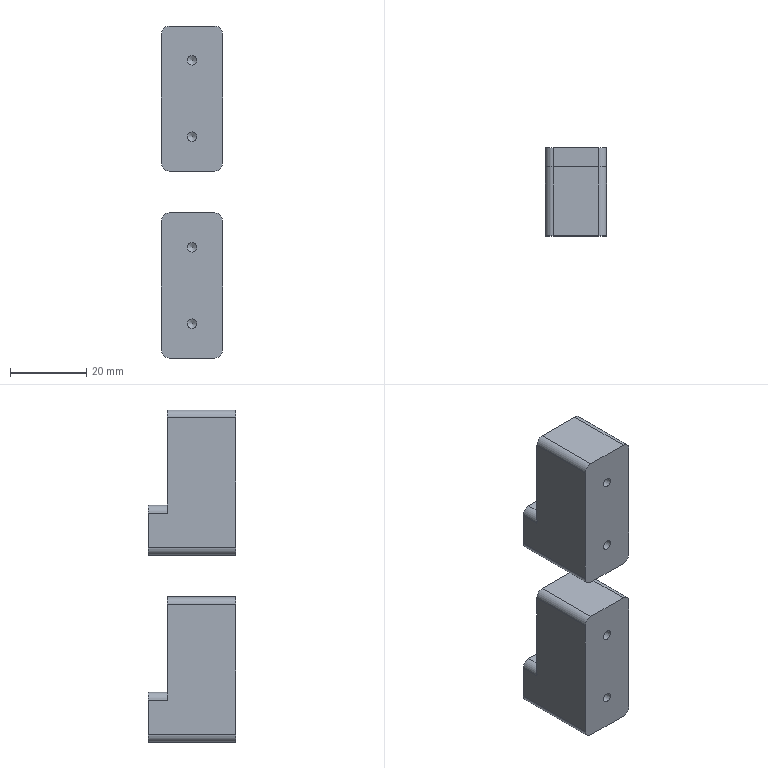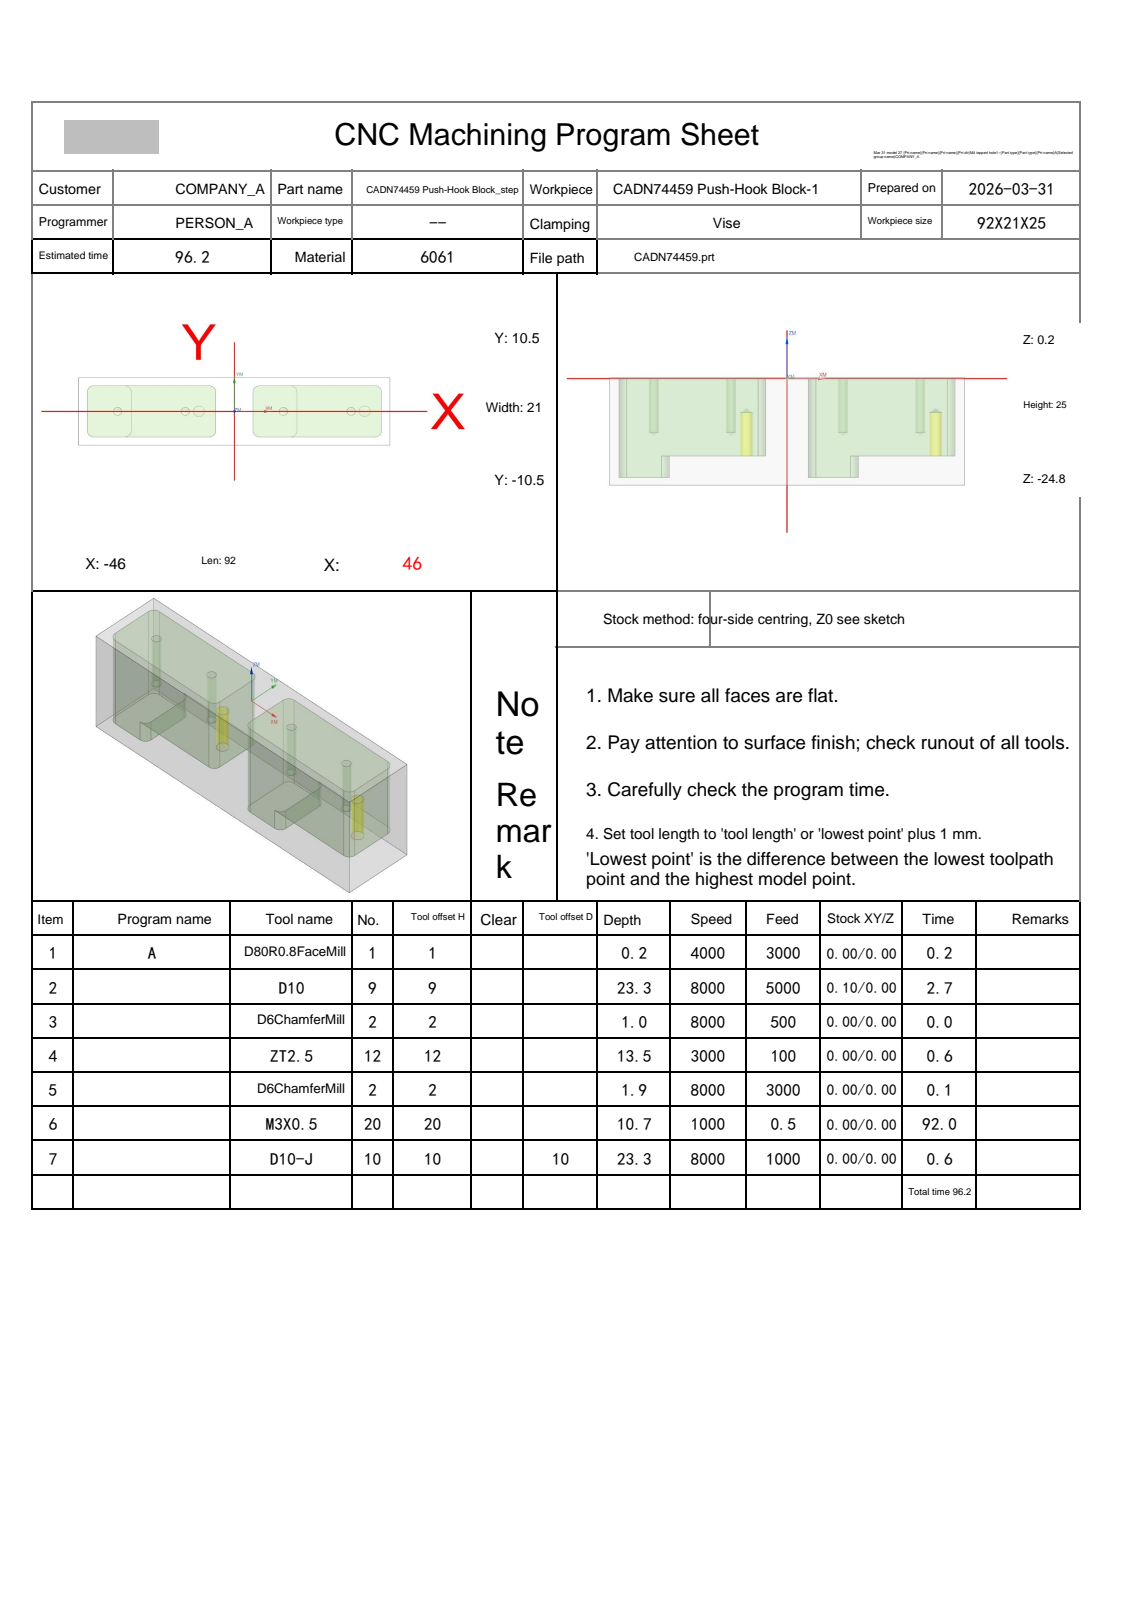NC program | NX | posted by the shop | part box 16 x 23 x 87 mm
Whole program:
%
O0001
(Machine time: 181.72 MIN)
(===Total Tool:6===)
(T1=D80R0.8 Mill D=80.  R=0.8  D-  H01 Z=0.    )
(T9=D10     D=10.  R=0.   D-  H09 Z=-23.1 )
(T2=D6ChamferMill   D=6.   R=0.   D-  H02 Z=-1.75 )
(T12=ZT2.5  D=2.5  DR_a=118 D-  H12 Z=-13.25)
(T20=M3X0.5 D=2.5  DR_a=180 D-  H20 Z=-10.5 )
(T10=D10-J  D=10.  R=0.   D10 H10 Z=-23.1 )
G80 G90 G17 G49 G40
G91 G28 Z0
M01
N1 T01 M06
(D80R0.8 Mill  D=80. R=0.8 H=01 ce=0.20 di=0.10)
G00 G90 G54 X-88.5 Y0.0 M03 S4000
G43 H01 Z20.
M08
Z2.1
G01 Z.1 F3000.
X-83.5
X83.5
X88.5
Z2.1
G00 Z20.
G00 G90 X-88.5 Y0.0 M03 S4000
Z20.
Z2.
G01 Z0.0 F1000.
X-83.5
X83.5
X88.5
Z2.
G00 Z20.
G91 G28 Z0.0
M05
M09
G91 G28 Z0.0
M01
N2 T09 M06
(D10  D=10. R=0. H=09 ce=0.10 di=0.00)
G00 G90 G54 X24.5 Y13.1 M03 S8000
G43 H09 Z20.
M08
Z.5
G01 X41.5 Z.439 F5000.
G02 X48.6 Y6. Z.399 I0.0 J-7.1
G01 Y-6. Z.355
G02 X41.5 Y-13.1 Z.315 I-7.1 J0.0
G01 X7.5 Z.193
G02 X.4 Y-6. Z.153 I0.0 J7.1
G01 Y6. Z.11
G02 X7.5 Y13.1 Z.07 I7.1 J0.0
G01 X41.5 Z-.053
G02 X48.6 Y6. Z-.093 I0.0 J-7.1
G01 Y-6. Z-.136
G02 X41.5 Y-13.1 Z-.176 I-7.1 J0.0
G01 X7.5 Z-.299
G02 X.4 Y-6. Z-.339 I0.0 J7.1
G01 Y6. Z-.382
G02 X7.5 Y13.1 Z-.422 I7.1 J0.0
G01 X41.5 Z-.545
G02 X48.6 Y6. Z-.585 I0.0 J-7.1
G01 Y-6. Z-.628
G02 X41.5 Y-13.1 Z-.668 I-7.1 J0.0
G01 X7.5 Z-.79
G02 X.4 Y-6. Z-.83 I0.0 J7.1
G01 Y6. Z-.874
G02 X7.5 Y13.1 Z-.914 I7.1 J0.0
G01 X41.5 Z-1.036
G02 X48.6 Y6. Z-1.076 I0.0 J-7.1
G01 Y-6. Z-1.12
G02 X41.5 Y-13.1 Z-1.16 I-7.1 J0.0
G01 X7.5 Z-1.282
G02 X.4 Y-6. Z-1.322 I0.0 J7.1
G01 Y6. Z-1.365
G02 X7.5 Y13.1 Z-1.405 I7.1 J0.0
G01 X41.5 Z-1.528
G02 X48.6 Y6. Z-1.568 I0.0 J-7.1
G01 Y-6. Z-1.611
G02 X41.5 Y-13.1 Z-1.651 I-7.1 J0.0
G01 X7.5 Z-1.774
G02 X.4 Y-6. Z-1.814 I0.0 J7.1
G01 Y6. Z-1.857
G02 X7.5 Y13.1 Z-1.897 I7.1 J0.0
G01 X41.5 Z-2.02
G02 X48.6 Y6. Z-2.06 I0.0 J-7.1
G01 Y-6. Z-2.103
G02 X41.5 Y-13.1 Z-2.143 I-7.1 J0.0
G01 X7.5 Z-2.265
G02 X.4 Y-6. Z-2.305 I0.0 J7.1
G01 Y6. Z-2.349
G02 X7.5 Y13.1 Z-2.389 I7.1 J0.0
G01 X41.5 Z-2.511
G02 X48.6 Y6. Z-2.551 I0.0 J-7.1
G01 Y-6. Z-2.595
G02 X41.5 Y-13.1 Z-2.635 I-7.1 J0.0
G01 X7.5 Z-2.757
G02 X.4 Y-6. Z-2.797 I0.0 J7.1
G01 Y6. Z-2.84
G02 X7.5 Y13.1 Z-2.88 I7.1 J0.0
G01 X41.5 Z-3.003
G02 X48.6 Y6. Z-3.043 I0.0 J-7.1
G01 Y-6. Z-3.086
G02 X41.5 Y-13.1 Z-3.126 I-7.1 J0.0
G01 X7.5 Z-3.249
G02 X.4 Y-6. Z-3.289 I0.0 J7.1
G01 Y6. Z-3.332
G02 X7.5 Y13.1 Z-3.372 I7.1 J0.0
G01 X41.5 Z-3.495
G02 X48.6 Y6. Z-3.535 I0.0 J-7.1
G01 Y-6. Z-3.578
G02 X41.5 Y-13.1 Z-3.618 I-7.1 J0.0
G01 X7.5 Z-3.74
G02 X.4 Y-6. Z-3.78 I0.0 J7.1
G01 Y6. Z-3.824
G02 X7.5 Y13.1 Z-3.864 I7.1 J0.0
G01 X41.5 Z-3.986
G02 X48.6 Y6. Z-4.026 I0.0 J-7.1
G01 Y-6. Z-4.07
G02 X41.5 Y-13.1 Z-4.11 I-7.1 J0.0
G01 X7.5 Z-4.232
G02 X.4 Y-6. Z-4.272 I0.0 J7.1
G01 Y6. Z-4.315
G02 X7.5 Y13.1 Z-4.355 I7.1 J0.0
G01 X41.5 Z-4.478
G02 X48.6 Y6. Z-4.518 I0.0 J-7.1
G01 Y-6. Z-4.561
G02 X41.5 Y-13.1 Z-4.601 I-7.1 J0.0
G01 X7.5 Z-4.724
G02 X.4 Y-6. Z-4.764 I0.0 J7.1
G01 Y6. Z-4.807
G02 X7.5 Y13.1 Z-4.847 I7.1 J0.0
G01 X41.5 Z-4.97
G02 X48.6 Y6. Z-5.01 I0.0 J-7.1
G01 Y-6. Z-5.053
G02 X41.5 Y-13.1 Z-5.093 I-7.1 J0.0
G01 X7.5 Z-5.215
G02 X.4 Y-6. Z-5.255 I0.0 J7.1
G01 Y6. Z-5.299
G02 X7.5 Y13.1 Z-5.339 I7.1 J0.0
G01 X41.5 Z-5.461
G02 X48.6 Y6. Z-5.501 I0.0 J-7.1
G01 Y-6. Z-5.545
G02 X41.5 Y-13.1 Z-5.585 I-7.1 J0.0
G01 X7.5 Z-5.707
G02 X.4 Y-6. Z-5.747 I0.0 J7.1
G01 Y6. Z-5.79
G02 X7.5 Y13.1 Z-5.83 I7.1 J0.0
G01 X41.5 Z-5.953
G02 X48.6 Y6. Z-5.993 I0.0 J-7.1
G01 Y-6. Z-6.036
G02 X41.5 Y-13.1 Z-6.076 I-7.1 J0.0
G01 X7.5 Z-6.199
G02 X.4 Y-6. Z-6.239 I0.0 J7.1
G01 Y6. Z-6.282
G02 X7.5 Y13.1 Z-6.322 I7.1 J0.0
G01 X41.5 Z-6.445
G02 X48.6 Y6. Z-6.485 I0.0 J-7.1
G01 Y-6. Z-6.528
G02 X41.5 Y-13.1 Z-6.568 I-7.1 J0.0
G01 X7.5 Z-6.69
G02 X.4 Y-6. Z-6.73 I0.0 J7.1
G01 Y6. Z-6.774
G02 X7.5 Y13.1 Z-6.814 I7.1 J0.0
G01 X41.5 Z-6.936
G02 X48.6 Y6. Z-6.976 I0.0 J-7.1
G01 Y-6. Z-7.02
G02 X41.5 Y-13.1 Z-7.06 I-7.1 J0.0
G01 X7.5 Z-7.182
G02 X.4 Y-6. Z-7.222 I0.0 J7.1
G01 Y6. Z-7.265
G02 X7.5 Y13.1 Z-7.305 I7.1 J0.0
G01 X41.5 Z-7.428
G02 X48.6 Y6. Z-7.468 I0.0 J-7.1
G01 Y-6. Z-7.511
G02 X41.5 Y-13.1 Z-7.551 I-7.1 J0.0
G01 X7.5 Z-7.674
G02 X.4 Y-6. Z-7.714 I0.0 J7.1
G01 Y6. Z-7.757
G02 X7.5 Y13.1 Z-7.797 I7.1 J0.0
G01 X41.5 Z-7.92
G02 X48.6 Y6. Z-7.96 I0.0 J-7.1
G01 Y-6. Z-8.003
G02 X41.5 Y-13.1 Z-8.043 I-7.1 J0.0
G01 X7.5 Z-8.165
G02 X.4 Y-6. Z-8.205 I0.0 J7.1
G01 Y6. Z-8.249
G02 X7.5 Y13.1 Z-8.289 I7.1 J0.0
G01 X41.5 Z-8.411
G02 X48.6 Y6. Z-8.451 I0.0 J-7.1
G01 Y-6. Z-8.495
G02 X41.5 Y-13.1 Z-8.535 I-7.1 J0.0
G01 X7.5 Z-8.657
G02 X.4 Y-6. Z-8.697 I0.0 J7.1
G01 Y6. Z-8.74
G02 X7.5 Y13.1 Z-8.78 I7.1 J0.0
G01 X41.5 Z-8.903
G02 X48.6 Y6. Z-8.943 I0.0 J-7.1
G01 Y-6. Z-8.986
G02 X41.5 Y-13.1 Z-9.026 I-7.1 J0.0
G01 X7.5 Z-9.149
G02 X.4 Y-6. Z-9.189 I0.0 J7.1
G01 Y6. Z-9.232
G02 X7.5 Y13.1 Z-9.272 I7.1 J0.0
G01 X41.5 Z-9.395
G02 X48.6 Y6. Z-9.435 I0.0 J-7.1
G01 Y-6. Z-9.478
G02 X41.5 Y-13.1 Z-9.518 I-7.1 J0.0
G01 X7.5 Z-9.64
G02 X.4 Y-6. Z-9.68 I0.0 J7.1
G01 Y6. Z-9.724
G02 X7.5 Y13.1 Z-9.764 I7.1 J0.0
G01 X41.5 Z-9.886
G02 X48.6 Y6. Z-9.926 I0.0 J-7.1
G01 Y-6. Z-9.97
G02 X41.5 Y-13.1 Z-10.01 I-7.1 J0.0
G01 X7.5 Z-10.132
G02 X.4 Y-6. Z-10.172 I0.0 J7.1
G01 Y6. Z-10.215
G02 X7.5 Y13.1 Z-10.255 I7.1 J0.0
G01 X41.5 Z-10.378
G02 X48.6 Y6. Z-10.418 I0.0 J-7.1
G01 Y-6. Z-10.461
G02 X41.5 Y-13.1 Z-10.501 I-7.1 J0.0
G01 X7.5 Z-10.624
G02 X.4 Y-6. Z-10.664 I0.0 J7.1
G01 Y6. Z-10.707
G02 X7.5 Y13.1 Z-10.747 I7.1 J0.0
G01 X41.5 Z-10.87
G02 X48.6 Y6. Z-10.91 I0.0 J-7.1
G01 Y-6. Z-10.953
G02 X41.5 Y-13.1 Z-10.993 I-7.1 J0.0
G01 X7.5 Z-11.115
G02 X.4 Y-6. Z-11.155 I0.0 J7.1
G01 Y6. Z-11.199
G02 X7.5 Y13.1 Z-11.239 I7.1 J0.0
G01 X41.5 Z-11.361
G02 X48.6 Y6. Z-11.401 I0.0 J-7.1
G01 Y-6. Z-11.445
G02 X41.5 Y-13.1 Z-11.485 I-7.1 J0.0
G01 X7.5 Z-11.607
G02 X.4 Y-6. Z-11.647 I0.0 J7.1
G01 Y6. Z-11.69
G02 X7.5 Y13.1 Z-11.73 I7.1 J0.0
G01 X41.5 Z-11.853
G02 X48.6 Y6. Z-11.893 I0.0 J-7.1
G01 Y-6. Z-11.936
G02 X41.5 Y-13.1 Z-11.976 I-7.1 J0.0
G01 X7.5 Z-12.099
G02 X.4 Y-6. Z-12.139 I0.0 J7.1
G01 Y6. Z-12.182
G02 X7.5 Y13.1 Z-12.222 I7.1 J0.0
G01 X41.5 Z-12.345
G02 X48.6 Y6. Z-12.385 I0.0 J-7.1
G01 Y-6. Z-12.428
G02 X41.5 Y-13.1 Z-12.468 I-7.1 J0.0
G01 X7.5 Z-12.59
G02 X.4 Y-6. Z-12.63 I0.0 J7.1
G01 Y6. Z-12.674
G02 X7.5 Y13.1 Z-12.714 I7.1 J0.0
G01 X41.5 Z-12.836
G02 X48.6 Y6. Z-12.876 I0.0 J-7.1
G01 Y-6. Z-12.92
G02 X41.5 Y-13.1 Z-12.96 I-7.1 J0.0
G01 X7.5 Z-13.082
G02 X.4 Y-6. Z-13.122 I0.0 J7.1
G01 Y6. Z-13.165
G02 X7.5 Y13.1 Z-13.205 I7.1 J0.0
G01 X41.5 Z-13.328
G02 X48.6 Y6. Z-13.368 I0.0 J-7.1
G01 Y-6. Z-13.411
G02 X41.5 Y-13.1 Z-13.451 I-7.1 J0.0
G01 X7.5 Z-13.574
G02 X.4 Y-6. Z-13.614 I0.0 J7.1
G01 Y6. Z-13.657
G02 X7.5 Y13.1 Z-13.697 I7.1 J0.0
G01 X41.5 Z-13.82
G02 X48.6 Y6. Z-13.86 I0.0 J-7.1
G01 Y-6. Z-13.903
G02 X41.5 Y-13.1 Z-13.943 I-7.1 J0.0
G01 X7.5 Z-14.065
G02 X.4 Y-6. Z-14.105 I0.0 J7.1
G01 Y6. Z-14.149
G02 X7.5 Y13.1 Z-14.189 I7.1 J0.0
G01 X41.5 Z-14.311
G02 X48.6 Y6. Z-14.351 I0.0 J-7.1
G01 Y-6. Z-14.395
G02 X41.5 Y-13.1 Z-14.435 I-7.1 J0.0
G01 X7.5 Z-14.557
G02 X.4 Y-6. Z-14.597 I0.0 J7.1
G01 Y6. Z-14.64
G02 X7.5 Y13.1 Z-14.68 I7.1 J0.0
G01 X41.5 Z-14.803
G02 X48.6 Y6. Z-14.843 I0.0 J-7.1
G01 Y-6. Z-14.886
G02 X41.5 Y-13.1 Z-14.926 I-7.1 J0.0
G01 X7.5 Z-15.049
G02 X.4 Y-6. Z-15.089 I0.0 J7.1
G01 Y6. Z-15.132
G02 X7.5 Y13.1 Z-15.172 I7.1 J0.0
G01 X41.5 Z-15.295
G02 X48.6 Y6. Z-15.335 I0.0 J-7.1
G01 Y-6. Z-15.378
G02 X41.5 Y-13.1 Z-15.418 I-7.1 J0.0
G01 X7.5 Z-15.54
G02 X.4 Y-6. Z-15.58 I0.0 J7.1
G01 Y6. Z-15.624
G02 X7.5 Y13.1 Z-15.664 I7.1 J0.0
G01 X41.5 Z-15.786
G02 X48.6 Y6. Z-15.826 I0.0 J-7.1
G01 Y-6. Z-15.87
G02 X41.5 Y-13.1 Z-15.91 I-7.1 J0.0
G01 X7.5 Z-16.032
G02 X.4 Y-6. Z-16.072 I0.0 J7.1
G01 Y6. Z-16.115
G02 X7.5 Y13.1 Z-16.155 I7.1 J0.0
G01 X41.5 Z-16.278
G02 X48.6 Y6. Z-16.318 I0.0 J-7.1
G01 Y-6. Z-16.361
G02 X41.5 Y-13.1 Z-16.401 I-7.1 J0.0
G01 X7.5 Z-16.524
G02 X.4 Y-6. Z-16.564 I0.0 J7.1
G01 Y6. Z-16.607
G02 X7.5 Y13.1 Z-16.647 I7.1 J0.0
G01 X41.5 Z-16.77
G02 X48.6 Y6. Z-16.81 I0.0 J-7.1
G01 Y-6. Z-16.853
G02 X41.5 Y-13.1 Z-16.893 I-7.1 J0.0
G01 X7.5 Z-17.015
G02 X.4 Y-6. Z-17.055 I0.0 J7.1
G01 Y6. Z-17.099
G02 X7.5 Y13.1 Z-17.139 I7.1 J0.0
G01 X41.5 Z-17.261
G02 X48.6 Y6. Z-17.301 I0.0 J-7.1
G01 Y-6. Z-17.345
G02 X41.5 Y-13.1 Z-17.385 I-7.1 J0.0
G01 X7.5 Z-17.507
G02 X.4 Y-6. Z-17.547 I0.0 J7.1
G01 Y6. Z-17.59
G02 X7.5 Y13.1 Z-17.63 I7.1 J0.0
G01 X41.5 Z-17.753
G02 X48.6 Y6. Z-17.793 I0.0 J-7.1
G01 Y-6. Z-17.836
G02 X41.5 Y-13.1 Z-17.876 I-7.1 J0.0
G01 X7.5 Z-17.999
G02 X.4 Y-6. Z-18.039 I0.0 J7.1
G01 Y6. Z-18.082
G02 X7.5 Y13.1 Z-18.122 I7.1 J0.0
G01 X41.5 Z-18.245
G02 X48.6 Y6. Z-18.285 I0.0 J-7.1
G01 Y-6. Z-18.328
G02 X41.5 Y-13.1 Z-18.368 I-7.1 J0.0
G01 X7.5 Z-18.49
G02 X.4 Y-6. Z-18.53 I0.0 J7.1
G01 Y6. Z-18.574
G02 X7.5 Y13.1 Z-18.614 I7.1 J0.0
G01 X41.5 Z-18.736
G02 X48.6 Y6. Z-18.776 I0.0 J-7.1
G01 Y-6. Z-18.82
G02 X41.5 Y-13.1 Z-18.86 I-7.1 J0.0
G01 X7.5 Z-18.982
G02 X.4 Y-6. Z-19.022 I0.0 J7.1
G01 Y6. Z-19.065
G02 X7.5 Y13.1 Z-19.105 I7.1 J0.0
G01 X41.5 Z-19.228
G02 X48.6 Y6. Z-19.268 I0.0 J-7.1
G01 Y-6. Z-19.311
G02 X41.5 Y-13.1 Z-19.351 I-7.1 J0.0
G01 X7.5 Z-19.474
G02 X.4 Y-6. Z-19.514 I0.0 J7.1
G01 Y6. Z-19.557
G02 X7.5 Y13.1 Z-19.597 I7.1 J0.0
G01 X41.5 Z-19.72
G02 X48.6 Y6. Z-19.76 I0.0 J-7.1
G01 Y-6. Z-19.803
G02 X41.5 Y-13.1 Z-19.843 I-7.1 J0.0
G01 X7.5 Z-19.965
G02 X.4 Y-6. Z-20.005 I0.0 J7.1
G01 Y6. Z-20.049
G02 X7.5 Y13.1 Z-20.089 I7.1 J0.0
G01 X41.5 Z-20.211
G02 X48.6 Y6. Z-20.251 I0.0 J-7.1
G01 Y-6. Z-20.295
G02 X41.5 Y-13.1 Z-20.335 I-7.1 J0.0
G01 X7.5 Z-20.457
G02 X.4 Y-6. Z-20.497 I0.0 J7.1
G01 Y6. Z-20.54
G02 X7.5 Y13.1 Z-20.58 I7.1 J0.0
G01 X41.5 Z-20.703
G02 X48.6 Y6. Z-20.743 I0.0 J-7.1
G01 Y-6. Z-20.786
G02 X41.5 Y-13.1 Z-20.826 I-7.1 J0.0
G01 X7.5 Z-20.949
G02 X.4 Y-6. Z-20.989 I0.0 J7.1
G01 Y6. Z-21.032
G02 X7.5 Y13.1 Z-21.072 I7.1 J0.0
G01 X41.5 Z-21.195
G02 X48.6 Y6. Z-21.235 I0.0 J-7.1
G01 Y-6. Z-21.278
G02 X41.5 Y-13.1 Z-21.318 I-7.1 J0.0
G01 X7.5 Z-21.44
G02 X.4 Y-6. Z-21.48 I0.0 J7.1
G01 Y6. Z-21.524
G02 X7.5 Y13.1 Z-21.564 I7.1 J0.0
G01 X41.5 Z-21.686
G02 X48.6 Y6. Z-21.726 I0.0 J-7.1
G01 Y-6. Z-21.77
G02 X41.5 Y-13.1 Z-21.81 I-7.1 J0.0
G01 X7.5 Z-21.932
G02 X.4 Y-6. Z-21.972 I0.0 J7.1
G01 Y6. Z-22.015
G02 X7.5 Y13.1 Z-22.055 I7.1 J0.0
G01 X41.5 Z-22.178
G02 X48.6 Y6. Z-22.218 I0.0 J-7.1
G01 Y-6. Z-22.261
G02 X41.5 Y-13.1 Z-22.301 I-7.1 J0.0
G01 X7.5 Z-22.424
G02 X.4 Y-6. Z-22.464 I0.0 J7.1
G01 Y6. Z-22.507
G02 X7.5 Y13.1 Z-22.547 I7.1 J0.0
G01 X41.5 Z-22.67
G02 X48.6 Y6. Z-22.71 I0.0 J-7.1
G01 Y-6. Z-22.753
G02 X41.5 Y-13.1 Z-22.793 I-7.1 J0.0
G01 X7.5 Z-22.915
G02 X.4 Y-6. Z-22.955 I0.0 J7.1
G01 Y6. Z-22.999
G02 X7.5 Y13.1 Z-23.039 I7.1 J0.0
G01 X24.5 Z-23.1
X41.5
G02 X48.6 Y6. I0.0 J-7.1
G01 Y-6.
G02 X41.5 Y-13.1 I-7.1 J0.0
G01 X7.5
G02 X.4 Y-6. I0.0 J7.1
G01 Y6.
G02 X7.5 Y13.1 I7.1 J0.0
G01 X24.5
X25.
Z-22.1
G00 Z20.
X-24.5
Z.5
G01 X-7.5 Z.439
G02 X-.4 Y6. Z.399 I0.0 J-7.1
G01 Y-6. Z.355
G02 X-7.5 Y-13.1 Z.315 I-7.1 J0.0
G01 X-41.5 Z.193
G02 X-48.6 Y-6. Z.153 I0.0 J7.1
G01 Y6. Z.11
G02 X-41.5 Y13.1 Z.07 I7.1 J0.0
G01 X-7.5 Z-.053
G02 X-.4 Y6. Z-.093 I0.0 J-7.1
G01 Y-6. Z-.136
G02 X-7.5 Y-13.1 Z-.176 I-7.1 J0.0
G01 X-41.5 Z-.299
G02 X-48.6 Y-6. Z-.339 I0.0 J7.1
G01 Y6. Z-.382
G02 X-41.5 Y13.1 Z-.422 I7.1 J0.0
G01 X-7.5 Z-.545
G02 X-.4 Y6. Z-.585 I0.0 J-7.1
G01 Y-6. Z-.628
G02 X-7.5 Y-13.1 Z-.668 I-7.1 J0.0
G01 X-41.5 Z-.79
G02 X-48.6 Y-6. Z-.83 I0.0 J7.1
G01 Y6. Z-.874
G02 X-41.5 Y13.1 Z-.914 I7.1 J0.0
G01 X-7.5 Z-1.036
G02 X-.4 Y6. Z-1.076 I0.0 J-7.1
G01 Y-6. Z-1.12
G02 X-7.5 Y-13.1 Z-1.16 I-7.1 J0.0
G01 X-41.5 Z-1.282
G02 X-48.6 Y-6. Z-1.322 I0.0 J7.1
G01 Y6. Z-1.365
G02 X-41.5 Y13.1 Z-1.405 I7.1 J0.0
G01 X-7.5 Z-1.528
G02 X-.4 Y6. Z-1.568 I0.0 J-7.1
G01 Y-6. Z-1.611
G02 X-7.5 Y-13.1 Z-1.651 I-7.1 J0.0
G01 X-41.5 Z-1.774
G02 X-48.6 Y-6. Z-1.814 I0.0 J7.1
G01 Y6. Z-1.857
G02 X-41.5 Y13.1 Z-1.897 I7.1 J0.0
G01 X-7.5 Z-2.02
G02 X-.4 Y6. Z-2.06 I0.0 J-7.1
G01 Y-6. Z-2.103
G02 X-7.5 Y-13.1 Z-2.143 I-7.1 J0.0
G01 X-41.5 Z-2.265
G02 X-48.6 Y-6. Z-2.305 I0.0 J7.1
G01 Y6. Z-2.349
G02 X-41.5 Y13.1 Z-2.389 I7.1 J0.0
G01 X-7.5 Z-2.511
G02 X-.4 Y6. Z-2.551 I0.0 J-7.1
G01 Y-6. Z-2.595
G02 X-7.5 Y-13.1 Z-2.635 I-7.1 J0.0
G01 X-41.5 Z-2.757
G02 X-48.6 Y-6. Z-2.797 I0.0 J7.1
G01 Y6. Z-2.84
G02 X-41.5 Y13.1 Z-2.88 I7.1 J0.0
G01 X-7.5 Z-3.003
G02 X-.4 Y6. Z-3.043 I0.0 J-7.1
G01 Y-6. Z-3.086
G02 X-7.5 Y-13.1 Z-3.126 I-7.1 J0.0
G01 X-41.5 Z-3.249
G02 X-48.6 Y-6. Z-3.289 I0.0 J7.1
G01 Y6. Z-3.332
G02 X-41.5 Y13.1 Z-3.372 I7.1 J0.0
G01 X-7.5 Z-3.495
G02 X-.4 Y6. Z-3.535 I0.0 J-7.1
G01 Y-6. Z-3.578
G02 X-7.5 Y-13.1 Z-3.618 I-7.1 J0.0
G01 X-41.5 Z-3.74
G02 X-48.6 Y-6. Z-3.78 I0.0 J7.1
G01 Y6. Z-3.824
G02 X-41.5 Y13.1 Z-3.864 I7.1 J0.0
G01 X-7.5 Z-3.986
G02 X-.4 Y6. Z-4.026 I0.0 J-7.1
G01 Y-6. Z-4.07
G02 X-7.5 Y-13.1 Z-4.11 I-7.1 J0.0
G01 X-41.5 Z-4.232
G02 X-48.6 Y-6. Z-4.272 I0.0 J7.1
G01 Y6. Z-4.315
G02 X-41.5 Y13.1 Z-4.355 I7.1 J0.0
G01 X-7.5 Z-4.478
G02 X-.4 Y6. Z-4.518 I0.0 J-7.1
G01 Y-6. Z-4.561
G02 X-7.5 Y-13.1 Z-4.601 I-7.1 J0.0
G01 X-41.5 Z-4.724
G02 X-48.6 Y-6. Z-4.764 I0.0 J7.1
G01 Y6. Z-4.807
G02 X-41.5 Y13.1 Z-4.847 I7.1 J0.0
G01 X-7.5 Z-4.97
G02 X-.4 Y6. Z-5.01 I0.0 J-7.1
G01 Y-6. Z-5.053
G02 X-7.5 Y-13.1 Z-5.093 I-7.1 J0.0
G01 X-41.5 Z-5.215
G02 X-48.6 Y-6. Z-5.255 I0.0 J7.1
G01 Y6. Z-5.299
G02 X-41.5 Y13.1 Z-5.339 I7.1 J0.0
G01 X-7.5 Z-5.461
G02 X-.4 Y6. Z-5.501 I0.0 J-7.1
G01 Y-6. Z-5.545
G02 X-7.5 Y-13.1 Z-5.585 I-7.1 J0.0
G01 X-41.5 Z-5.707
G02 X-48.6 Y-6. Z-5.747 I0.0 J7.1
G01 Y6. Z-5.79
G02 X-41.5 Y13.1 Z-5.83 I7.1 J0.0
G01 X-7.5 Z-5.953
G02 X-.4 Y6. Z-5.993 I0.0 J-7.1
G01 Y-6. Z-6.036
G02 X-7.5 Y-13.1 Z-6.076 I-7.1 J0.0
G01 X-41.5 Z-6.199
G02 X-48.6 Y-6. Z-6.239 I0.0 J7.1
G01 Y6. Z-6.282
G02 X-41.5 Y13.1 Z-6.322 I7.1 J0.0
G01 X-7.5 Z-6.445
G02 X-.4 Y6. Z-6.485 I0.0 J-7.1
G01 Y-6. Z-6.528
G02 X-7.5 Y-13.1 Z-6.568 I-7.1 J0.0
G01 X-41.5 Z-6.69
G02 X-48.6 Y-6. Z-6.73 I0.0 J7.1
G01 Y6. Z-6.774
G02 X-41.5 Y13.1 Z-6.814 I7.1 J0.0
G01 X-7.5 Z-6.936
G02 X-.4 Y6. Z-6.976 I0.0 J-7.1
G01 Y-6. Z-7.02
G02 X-7.5 Y-13.1 Z-7.06 I-7.1 J0.0
G01 X-41.5 Z-7.182
G02 X-48.6 Y-6. Z-7.222 I0.0 J7.1
G01 Y6. Z-7.265
G02 X-41.5 Y13.1 Z-7.305 I7.1 J0.0
G01 X-7.5 Z-7.428
G02 X-.4 Y6. Z-7.468 I0.0 J-7.1
G01 Y-6. Z-7.511
G02 X-7.5 Y-13.1 Z-7.551 I-7.1 J0.0
G01 X-41.5 Z-7.674
G02 X-48.6 Y-6. Z-7.714 I0.0 J7.1
G01 Y6. Z-7.757
G02 X-41.5 Y13.1 Z-7.797 I7.1 J0.0
G01 X-7.5 Z-7.92
G02 X-.4 Y6. Z-7.96 I0.0 J-7.1
G01 Y-6. Z-8.003
G02 X-7.5 Y-13.1 Z-8.043 I-7.1 J0.0
G01 X-41.5 Z-8.165
G02 X-48.6 Y-6. Z-8.205 I0.0 J7.1
G01 Y6. Z-8.249
G02 X-41.5 Y13.1 Z-8.289 I7.1 J0.0
G01 X-7.5 Z-8.411
G02 X-.4 Y6. Z-8.451 I0.0 J-7.1
G01 Y-6. Z-8.495
G02 X-7.5 Y-13.1 Z-8.535 I-7.1 J0.0
G01 X-41.5 Z-8.657
G02 X-48.6 Y-6. Z-8.697 I0.0 J7.1
G01 Y6. Z-8.74
G02 X-41.5 Y13.1 Z-8.78 I7.1 J0.0
G01 X-7.5 Z-8.903
G02 X-.4 Y6. Z-8.943 I0.0 J-7.1
G01 Y-6. Z-8.986
G02 X-7.5 Y-13.1 Z-9.026 I-7.1 J0.0
G01 X-41.5 Z-9.149
G02 X-48.6 Y-6. Z-9.189 I0.0 J7.1
G01 Y6. Z-9.232
G02 X-41.5 Y13.1 Z-9.272 I7.1 J0.0
G01 X-7.5 Z-9.395
G02 X-.4 Y6. Z-9.435 I0.0 J-7.1
G01 Y-6. Z-9.478
G02 X-7.5 Y-13.1 Z-9.518 I-7.1 J0.0
G01 X-41.5 Z-9.64
G02 X-48.6 Y-6. Z-9.68 I0.0 J7.1
G01 Y6. Z-9.724
G02 X-41.5 Y13.1 Z-9.764 I7.1 J0.0
G01 X-7.5 Z-9.886
G02 X-.4 Y6. Z-9.926 I0.0 J-7.1
G01 Y-6. Z-9.97
G02 X-7.5 Y-13.1 Z-10.01 I-7.1 J0.0
G01 X-41.5 Z-10.132
G02 X-48.6 Y-6. Z-10.172 I0.0 J7.1
G01 Y6. Z-10.215
G02 X-41.5 Y13.1 Z-10.255 I7.1 J0.0
G01 X-7.5 Z-10.378
G02 X-.4 Y6. Z-10.418 I0.0 J-7.1
G01 Y-6. Z-10.461
G02 X-7.5 Y-13.1 Z-10.501 I-7.1 J0.0
G01 X-41.5 Z-10.624
G02 X-48.6 Y-6. Z-10.664 I0.0 J7.1
G01 Y6. Z-10.707
G02 X-41.5 Y13.1 Z-10.747 I7.1 J0.0
G01 X-7.5 Z-10.87
G02 X-.4 Y6. Z-10.91 I0.0 J-7.1
G01 Y-6. Z-10.953
G02 X-7.5 Y-13.1 Z-10.993 I-7.1 J0.0
G01 X-41.5 Z-11.115
G02 X-48.6 Y-6. Z-11.155 I0.0 J7.1
G01 Y6. Z-11.199
G02 X-41.5 Y13.1 Z-11.239 I7.1 J0.0
G01 X-7.5 Z-11.361
G02 X-.4 Y6. Z-11.401 I0.0 J-7.1
G01 Y-6. Z-11.445
G02 X-7.5 Y-13.1 Z-11.485 I-7.1 J0.0
G01 X-41.5 Z-11.607
G02 X-48.6 Y-6. Z-11.647 I0.0 J7.1
G01 Y6. Z-11.69
G02 X-41.5 Y13.1 Z-11.73 I7.1 J0.0
G01 X-7.5 Z-11.853
G02 X-.4 Y6. Z-11.893 I0.0 J-7.1
G01 Y-6. Z-11.936
G02 X-7.5 Y-13.1 Z-11.976 I-7.1 J0.0
G01 X-41.5 Z-12.099
G02 X-48.6 Y-6. Z-12.139 I0.0 J7.1
G01 Y6. Z-12.182
G02 X-41.5 Y13.1 Z-12.222 I7.1 J0.0
G01 X-7.5 Z-12.345
G02 X-.4 Y6. Z-12.385 I0.0 J-7.1
G01 Y-6. Z-12.428
G02 X-7.5 Y-13.1 Z-12.468 I-7.1 J0.0
G01 X-41.5 Z-12.59
G02 X-48.6 Y-6. Z-12.63 I0.0 J7.1
G01 Y6. Z-12.674
G02 X-41.5 Y13.1 Z-12.714 I7.1 J0.0
G01 X-7.5 Z-12.836
G02 X-.4 Y6. Z-12.876 I0.0 J-7.1
G01 Y-6. Z-12.92
G02 X-7.5 Y-13.1 Z-12.96 I-7.1 J0.0
G01 X-41.5 Z-13.082
G02 X-48.6 Y-6. Z-13.122 I0.0 J7.1
G01 Y6. Z-13.165
G02 X-41.5 Y13.1 Z-13.205 I7.1 J0.0
G01 X-7.5 Z-13.328
G02 X-.4 Y6. Z-13.368 I0.0 J-7.1
G01 Y-6. Z-13.411
G02 X-7.5 Y-13.1 Z-13.451 I-7.1 J0.0
G01 X-41.5 Z-13.574
G02 X-48.6 Y-6. Z-13.614 I0.0 J7.1
G01 Y6. Z-13.657
G02 X-41.5 Y13.1 Z-13.697 I7.1 J0.0
G01 X-7.5 Z-13.82
G02 X-.4 Y6. Z-13.86 I0.0 J-7.1
G01 Y-6. Z-13.903
G02 X-7.5 Y-13.1 Z-13.943 I-7.1 J0.0
G01 X-41.5 Z-14.065
G02 X-48.6 Y-6. Z-14.105 I0.0 J7.1
G01 Y6. Z-14.149
G02 X-41.5 Y13.1 Z-14.189 I7.1 J0.0
G01 X-7.5 Z-14.311
G02 X-.4 Y6. Z-14.351 I0.0 J-7.1
G01 Y-6. Z-14.395
G02 X-7.5 Y-13.1 Z-14.435 I-7.1 J0.0
G01 X-41.5 Z-14.557
G02 X-48.6 Y-6. Z-14.597 I0.0 J7.1
G01 Y6. Z-14.64
G02 X-41.5 Y13.1 Z-14.68 I7.1 J0.0
G01 X-7.5 Z-14.803
G02 X-.4 Y6. Z-14.843 I0.0 J-7.1
G01 Y-6. Z-14.886
G02 X-7.5 Y-13.1 Z-14.926 I-7.1 J0.0
G01 X-41.5 Z-15.049
G02 X-48.6 Y-6. Z-15.089 I0.0 J7.1
G01 Y6. Z-15.132
G02 X-41.5 Y13.1 Z-15.172 I7.1 J0.0
G01 X-7.5 Z-15.295
G02 X-.4 Y6. Z-15.335 I0.0 J-7.1
G01 Y-6. Z-15.378
G02 X-7.5 Y-13.1 Z-15.418 I-7.1 J0.0
G01 X-41.5 Z-15.54
G02 X-48.6 Y-6. Z-15.58 I0.0 J7.1
G01 Y6. Z-15.624
G02 X-41.5 Y13.1 Z-15.664 I7.1 J0.0
G01 X-7.5 Z-15.786
G02 X-.4 Y6. Z-15.826 I0.0 J-7.1
G01 Y-6. Z-15.87
G02 X-7.5 Y-13.1 Z-15.91 I-7.1 J0.0
G01 X-41.5 Z-16.032
G02 X-48.6 Y-6. Z-16.072 I0.0 J7.1
G01 Y6. Z-16.115
G02 X-41.5 Y13.1 Z-16.155 I7.1 J0.0
G01 X-7.5 Z-16.278
G02 X-.4 Y6. Z-16.318 I0.0 J-7.1
G01 Y-6. Z-16.361
G02 X-7.5 Y-13.1 Z-16.401 I-7.1 J0.0
G01 X-41.5 Z-16.524
G02 X-48.6 Y-6. Z-16.564 I0.0 J7.1
G01 Y6. Z-16.607
G02 X-41.5 Y13.1 Z-16.647 I7.1 J0.0
G01 X-7.5 Z-16.77
G02 X-.4 Y6. Z-16.81 I0.0 J-7.1
G01 Y-6. Z-16.853
G02 X-7.5 Y-13.1 Z-16.893 I-7.1 J0.0
G01 X-41.5 Z-17.015
G02 X-48.6 Y-6. Z-17.055 I0.0 J7.1
G01 Y6. Z-17.099
G02 X-41.5 Y13.1 Z-17.139 I7.1 J0.0
G01 X-7.5 Z-17.261
G02 X-.4 Y6. Z-17.301 I0.0 J-7.1
G01 Y-6. Z-17.345
G02 X-7.5 Y-13.1 Z-17.385 I-7.1 J0.0
G01 X-41.5 Z-17.507
G02 X-48.6 Y-6. Z-17.547 I0.0 J7.1
G01 Y6. Z-17.59
G02 X-41.5 Y13.1 Z-17.63 I7.1 J0.0
G01 X-7.5 Z-17.753
G02 X-.4 Y6. Z-17.793 I0.0 J-7.1
G01 Y-6. Z-17.836
G02 X-7.5 Y-13.1 Z-17.876 I-7.1 J0.0
G01 X-41.5 Z-17.999
G02 X-48.6 Y-6. Z-18.039 I0.0 J7.1
G01 Y6. Z-18.082
G02 X-41.5 Y13.1 Z-18.122 I7.1 J0.0
G01 X-7.5 Z-18.245
G02 X-.4 Y6. Z-18.285 I0.0 J-7.1
G01 Y-6. Z-18.328
G02 X-7.5 Y-13.1 Z-18.368 I-7.1 J0.0
G01 X-41.5 Z-18.49
G02 X-48.6 Y-6. Z-18.53 I0.0 J7.1
G01 Y6. Z-18.574
G02 X-41.5 Y13.1 Z-18.614 I7.1 J0.0
G01 X-7.5 Z-18.736
G02 X-.4 Y6. Z-18.776 I0.0 J-7.1
G01 Y-6. Z-18.82
G02 X-7.5 Y-13.1 Z-18.86 I-7.1 J0.0
G01 X-41.5 Z-18.982
G02 X-48.6 Y-6. Z-19.022 I0.0 J7.1
G01 Y6. Z-19.065
G02 X-41.5 Y13.1 Z-19.105 I7.1 J0.0
G01 X-7.5 Z-19.228
G02 X-.4 Y6. Z-19.268 I0.0 J-7.1
G01 Y-6. Z-19.311
G02 X-7.5 Y-13.1 Z-19.351 I-7.1 J0.0
G01 X-41.5 Z-19.474
G02 X-48.6 Y-6. Z-19.514 I0.0 J7.1
G01 Y6. Z-19.557
G02 X-41.5 Y13.1 Z-19.597 I7.1 J0.0
G01 X-7.5 Z-19.72
G02 X-.4 Y6. Z-19.76 I0.0 J-7.1
G01 Y-6. Z-19.803
G02 X-7.5 Y-13.1 Z-19.843 I-7.1 J0.0
G01 X-41.5 Z-19.965
G02 X-48.6 Y-6. Z-20.005 I0.0 J7.1
G01 Y6. Z-20.049
G02 X-41.5 Y13.1 Z-20.089 I7.1 J0.0
G01 X-7.5 Z-20.211
G02 X-.4 Y6. Z-20.251 I0.0 J-7.1
G01 Y-6. Z-20.295
G02 X-7.5 Y-13.1 Z-20.335 I-7.1 J0.0
G01 X-41.5 Z-20.457
G02 X-48.6 Y-6. Z-20.497 I0.0 J7.1
G01 Y6. Z-20.54
G02 X-41.5 Y13.1 Z-20.58 I7.1 J0.0
G01 X-7.5 Z-20.703
G02 X-.4 Y6. Z-20.743 I0.0 J-7.1
G01 Y-6. Z-20.786
G02 X-7.5 Y-13.1 Z-20.826 I-7.1 J0.0
G01 X-41.5 Z-20.949
G02 X-48.6 Y-6. Z-20.989 I0.0 J7.1
G01 Y6. Z-21.032
G02 X-41.5 Y13.1 Z-21.072 I7.1 J0.0
G01 X-7.5 Z-21.195
G02 X-.4 Y6. Z-21.235 I0.0 J-7.1
G01 Y-6. Z-21.278
G02 X-7.5 Y-13.1 Z-21.318 I-7.1 J0.0
G01 X-41.5 Z-21.44
G02 X-48.6 Y-6. Z-21.48 I0.0 J7.1
G01 Y6. Z-21.524
G02 X-41.5 Y13.1 Z-21.564 I7.1 J0.0
G01 X-7.5 Z-21.686
G02 X-.4 Y6. Z-21.726 I0.0 J-7.1
G01 Y-6. Z-21.77
G02 X-7.5 Y-13.1 Z-21.81 I-7.1 J0.0
G01 X-41.5 Z-21.932
G02 X-48.6 Y-6. Z-21.972 I0.0 J7.1
G01 Y6. Z-22.015
G02 X-41.5 Y13.1 Z-22.055 I7.1 J0.0
G01 X-7.5 Z-22.178
G02 X-.4 Y6. Z-22.218 I0.0 J-7.1
G01 Y-6. Z-22.261
G02 X-7.5 Y-13.1 Z-22.301 I-7.1 J0.0
G01 X-41.5 Z-22.424
G02 X-48.6 Y-6. Z-22.464 I0.0 J7.1
G01 Y6. Z-22.507
G02 X-41.5 Y13.1 Z-22.547 I7.1 J0.0
G01 X-7.5 Z-22.67
G02 X-.4 Y6. Z-22.71 I0.0 J-7.1
G01 Y-6. Z-22.753
G02 X-7.5 Y-13.1 Z-22.793 I-7.1 J0.0
G01 X-41.5 Z-22.915
G02 X-48.6 Y-6. Z-22.955 I0.0 J7.1
G01 Y6. Z-22.999
G02 X-41.5 Y13.1 Z-23.039 I7.1 J0.0
G01 X-24.5 Z-23.1
X-7.5
G02 X-.4 Y6. I0.0 J-7.1
G01 Y-6.
G02 X-7.5 Y-13.1 I-7.1 J0.0
G01 X-41.5
G02 X-48.6 Y-6. I0.0 J7.1
G01 Y6.
G02 X-41.5 Y13.1 I7.1 J0.0
G01 X-24.5
X-24.
Z-22.1
G00 Z20.
G91 G28 Z0.0
M05
M09
G91 G28 Z0.0
M01
N3 T02 M06
(D6ChamferMill  D=6. R=0. H=02 ce=0.00 di=0.00)
G00 G90 G54 X-34.5 Y0.0 M03 S8000
G43 H02 Z20.
M08
G98 G81 X-34.5 Y0.0 Z-.8 R1. F500.
X-14.5
X14.5
X34.5
G80
G00 Z20.
G91 G28 Z0.0
M05
M09
G91 G28 Z0.0
M01
N4 T12 M06
(ZT2.5 D=2.5 DR_a=118 H=12)
G00 G90 G54 X-34.5 Y0.0 M03 S3000
G43 H12 Z20.
M08
G98 G83 X-34.5 Y0.0 Z-13.251 R1. F100. Q2.
X-14.5
X14.5
X34.5
G80
G00 Z20.
G91 G28 Z0.0
M05
M09
G91 G28 Z0.0
M01
N5 T02 M06
(D6ChamferMill  D=6. R=0. H=02 ce=0.00 di=0.00)
G00 G90 G54 X-24.75 Y10.128 M03 S8000
G43 H02 Z20.
M08
Z2.099
G01 Z-1.5 F3000.
G03 X-24.83 Y9.828 I.52 J-.3
X-24.53 Y9.308 I.6 J0.0
G01 X-24.5 Y9.3
X-7.5
G02 X-4.2 Y6. I0.0 J-3.3
G01 Y-6.
G02 X-7.5 Y-9.3 I-3.3 J0.0
G01 X-41.5
G02 X-44.8 Y-6. I0.0 J3.3
G01 Y6.
G02 X-41.5 Y9.3 I3.3 J0.0
G01 X-24.5
X-24.47 Y9.308
G03 X-24.17 Y9.828 I-.3 J.52
X-24.25 Y10.128 I-.6 J0.0
G01 Z2.099
G00 Z20.
X24.25
Z2.099
G01 Z-1.5
G03 X24.17 Y9.828 I.52 J-.3
X24.47 Y9.308 I.6 J0.0
G01 X24.5 Y9.3
X41.5
G02 X44.8 Y6. I0.0 J-3.3
G01 Y-6.
G02 X41.5 Y-9.3 I-3.3 J0.0
G01 X7.5
G02 X4.2 Y-6. I0.0 J3.3
G01 Y6.
G02 X7.5 Y9.3 I3.3 J0.0
G01 X24.5
X24.53 Y9.308
G03 X24.83 Y9.828 I-.3 J.52
X24.75 Y10.128 I-.6 J0.0
G01 Z2.099
G00 Z20.
G00 G90 X-34.5 Y0.0 M03 S8000
Z20.
G98 G81 X-34.5 Y0.0 Z-1.75 R3. F500.
X-14.5
X14.5
X34.5
G80
G00 Z20.
G91 G28 Z0.0
M05
M09
G91 G28 Z0.0
M01
N6 T20 M06
(M3X0.5 D=2.5 DR_a=180 H=20)
G00 G90 G54 X-34.5 Y0.0 M03 S1000
G43 H20 Z20.
M08
G95
G98 G84 X-34.5 Y0.0 Z-10.5 R1. F.5 Q2.
X-14.5
X14.5
X34.5
G80
G94
G00 Z20.
G91 G28 Z0.0
M05
M09
G91 G28 Z0.0
M01
N7 T10 M06
(D10-J  D=10. R=0. H=10 ce=0.00 di=0.00)
G00 G90 G54 X-6.489 Y-14.137 M03 S8000
G43 H10 Z20.
M08
Z-11.05
G01 Z-11.55 F1000.
G41 D10
X-6.502 Y-13.938
G03 X-7.5 Y-13. I-.998 J-.063
G01 X-41.5
G02 X-48.5 Y-6. I0.0 J7.
G01 Y6.
G02 X-41.5 Y13. I7. J0.0
G01 X-7.5
G02 X-.5 Y6. I0.0 J-7.
G01 Y-6.
G02 X-7.5 Y-13. I-7. J0.0
G01 X-8.
G03 X-9. Y-14. I0.0 J-1.
G01 G40 Y-14.2
X.554 Y-10.357
G41 D10
X.729 Y-10.261
G03 X1.251 Y-9.383 I-.479 J.878
X1.157 Y-8.96 I-1. J0.0
G02 X.5 Y-6. I6.343 J2.96
G01 Y6.
G02 X7.5 Y13. I7. J0.0
G01 X41.5
G02 X48.5 Y6. I0.0 J-7.
G01 Y-6.
G02 X41.5 Y-13. I-7. J0.0
G01 X7.5
G02 X1.157 Y-8.96 I0.0 J7.
X.962 Y-8.5 I6.343 J2.96
G03 X.028 Y-7.857 I-.934 J-.357
X-.33 Y-7.923 I0.0 J-1.
G01 G40 X0.0 Y-8.784
Z-11.05
G00 Z20.
X-6.489 Y-14.137
Z-22.6
G01 Z-23.1
G41 D10
X-6.502 Y-13.938
G03 X-7.5 Y-13. I-.998 J-.063
G01 X-41.5
G02 X-48.5 Y-6. I0.0 J7.
G01 Y6.
G02 X-41.5 Y13. I7. J0.0
G01 X-7.5
G02 X-.5 Y6. I0.0 J-7.
G01 Y-6.
G02 X-7.5 Y-13. I-7. J0.0
G01 X-8.
G03 X-9. Y-14. I0.0 J-1.
G01 G40 Y-14.2
X.554 Y-10.357
G41 D10
X.729 Y-10.261
G03 X1.251 Y-9.383 I-.479 J.878
X1.157 Y-8.96 I-1. J0.0
G02 X.5 Y-6. I6.343 J2.96
G01 Y6.
G02 X7.5 Y13. I7. J0.0
G01 X41.5
G02 X48.5 Y6. I0.0 J-7.
G01 Y-6.
G02 X41.5 Y-13. I-7. J0.0
G01 X7.5
G02 X1.157 Y-8.96 I0.0 J7.
X.962 Y-8.5 I6.343 J2.96
G03 X.028 Y-7.857 I-.934 J-.357
X-.33 Y-7.923 I0.0 J-1.
G01 G40 X0.0 Y-8.784
Z-22.6
G00 Z20.
M05
M09
G91 G28 Z0.0
G91 G28 Y0.0
M30
%